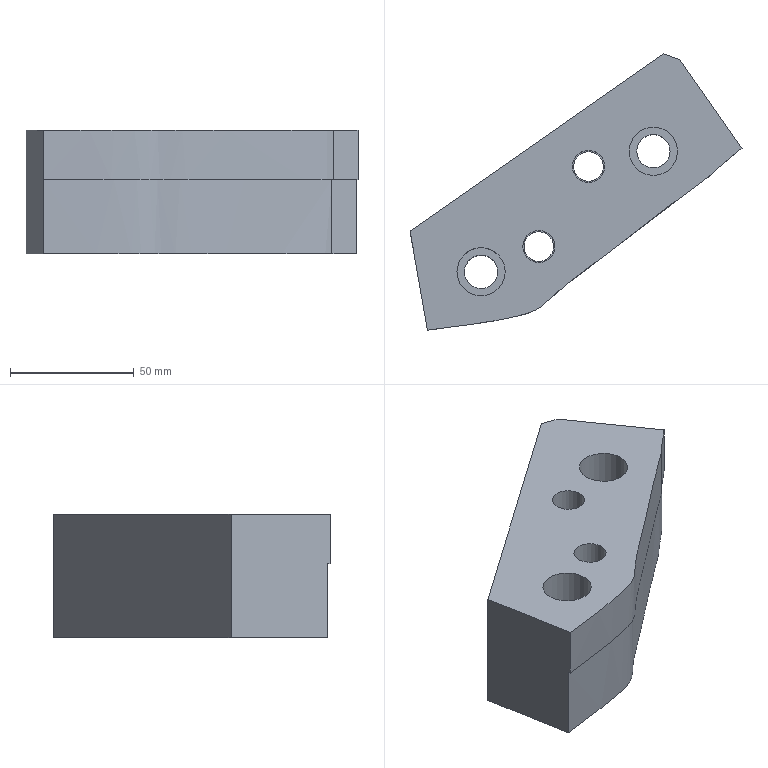Part | NX | features solid 2 | 1 solid | 23 faces | box 134.129 x 111.662 x 50 mm | volume 319985 mm3 | plane 13 | cylinder 8 | spline 2 | commonest cylinder face diameters 12 x2 13 x2 13.5 x2 19.5 x2
STEP:
#1=CARTESIAN_POINT('',(397.794,3.938,0.));
#2=VERTEX_POINT('',#1);
#3=CARTESIAN_POINT('',(397.794,3.938,-20.));
#4=VERTEX_POINT('',#3);
#5=CARTESIAN_POINT('',(397.794,3.938,-10.));
#6=DIRECTION('',(0.,0.,-1.));
#7=VECTOR('',#6,1000.);
#8=LINE('',#5,#7);
#9=EDGE_CURVE('',#2,#4,#8,.T.);
#10=ORIENTED_EDGE('',*,*,#9,.F.);
#11=CARTESIAN_POINT('',(280.528,-61.349,0.));
#12=VERTEX_POINT('',#11);
#13=CARTESIAN_POINT('',(397.794,3.938,0.));
#14=CARTESIAN_POINT('',(396.897,2.818,0.));
#15=CARTESIAN_POINT('',(394.657,0.9582,0.));
#16=CARTESIAN_POINT('',(391.166,-1.547,0.));
#17=CARTESIAN_POINT('',(387.681,-4.089,0.));
#18=CARTESIAN_POINT('',(383.042,-7.479,0.));
#19=CARTESIAN_POINT('',(377.298,-11.791,0.));
#20=CARTESIAN_POINT('',(370.456,-17.031,0.));
#21=CARTESIAN_POINT('',(363.642,-22.308,0.));
#22=CARTESIAN_POINT('',(356.835,-27.594,0.));
#23=CARTESIAN_POINT('',(350.02,-32.87,0.));
#24=CARTESIAN_POINT('',(344.299,-37.211,0.));
#25=CARTESIAN_POINT('',(339.673,-40.62,0.));
#26=CARTESIAN_POINT('',(336.169,-43.134,0.));
#27=CARTESIAN_POINT('',(332.961,-46.001,0.));
#28=CARTESIAN_POINT('',(329.879,-49.024,0.));
#29=CARTESIAN_POINT('',(326.665,-51.86,0.));
#30=CARTESIAN_POINT('',(322.954,-54.002,0.));
#31=CARTESIAN_POINT('',(318.75,-55.232,0.));
#32=CARTESIAN_POINT('',(314.576,-56.215,0.));
#33=CARTESIAN_POINT('',(310.363,-57.101,0.));
#34=CARTESIAN_POINT('',(304.716,-58.092,0.));
#35=CARTESIAN_POINT('',(297.617,-59.134,0.));
#36=CARTESIAN_POINT('',(289.07,-60.222,0.));
#37=CARTESIAN_POINT('',(283.374,-60.967,0.));
#38=CARTESIAN_POINT('',(280.528,-61.349,0.));
#39=B_SPLINE_CURVE_WITH_KNOTS('',3,(#13,#14,#15,#16,#17,#18,#19,#20,#21,#22,#23,#24,#25,#26,#27,#28,#29,#30,#31,#32,#33,#34,#35,#36,#37,#38),.UNSPECIFIED.,.F.,.F.,(4,1,1,1,1,1,1,1,1,1,1,1,1,1,1,1,1,1,1,1,1,1,1,4),(-0.08488,-0.08063,-0.07637,-0.07212,-0.06787,-0.05936,-0.05085,-0.04234,-0.03384,-0.02533,-0.01682,-0.01257,-0.008314,-0.004061,0.0001929,0.004447,0.0087,0.01295,0.01721,0.02146,0.02571,0.03422,0.04273,0.05124),.UNSPECIFIED.);
#40=EDGE_CURVE('',#2,#12,#39,.T.);
#41=ORIENTED_EDGE('',*,*,#40,.T.);
#42=CARTESIAN_POINT('',(280.528,-61.349,-20.));
#43=VERTEX_POINT('',#42);
#44=CARTESIAN_POINT('',(280.528,-61.349,-10.));
#45=DIRECTION('',(0.,0.,-1.));
#46=VECTOR('',#45,1000.);
#47=LINE('',#44,#46);
#48=EDGE_CURVE('',#12,#43,#47,.T.);
#49=ORIENTED_EDGE('',*,*,#48,.T.);
#50=CARTESIAN_POINT('',(-190.231,-121.49,-20.));
#51=CARTESIAN_POINT('',(-188.654,-121.152,-20.));
#52=CARTESIAN_POINT('',(-185.47,-120.627,-20.));
#53=CARTESIAN_POINT('',(-180.656,-120.141,-20.));
#54=CARTESIAN_POINT('',(-175.882,-119.326,-20.));
#55=CARTESIAN_POINT('',(-169.679,-117.528,-20.));
#56=CARTESIAN_POINT('',(-162.185,-114.539,-20.));
#57=CARTESIAN_POINT('',(-153.086,-111.254,-20.));
#58=CARTESIAN_POINT('',(-144.031,-107.845,-20.));
#59=CARTESIAN_POINT('',(-136.465,-105.061,-20.));
#60=CARTESIAN_POINT('',(-130.418,-102.814,-20.));
#61=CARTESIAN_POINT('',(-125.812,-101.329,-20.));
#62=CARTESIAN_POINT('',(-121.306,-99.566,-20.));
#63=CARTESIAN_POINT('',(-116.876,-97.626,-20.));
#64=CARTESIAN_POINT('',(-112.335,-95.923,-20.));
#65=CARTESIAN_POINT('',(-107.564,-95.05,-20.));
#66=CARTESIAN_POINT('',(-102.756,-94.525,-20.));
#67=CARTESIAN_POINT('',(-96.349,-93.771,-20.));
#68=CARTESIAN_POINT('',(-89.902,-93.468,-20.));
#69=CARTESIAN_POINT('',(-83.452,-93.448,-20.));
#70=CARTESIAN_POINT('',(-77.002,-93.469,-20.));
#71=CARTESIAN_POINT('',(-68.939,-93.411,-20.));
#72=CARTESIAN_POINT('',(-56.04,-93.3,-20.));
#73=CARTESIAN_POINT('',(-33.465,-93.184,-20.));
#74=CARTESIAN_POINT('',(-7.666,-93.074,-20.));
#75=CARTESIAN_POINT('',(14.907,-92.653,-20.));
#76=CARTESIAN_POINT('',(27.794,-92.068,-20.));
#77=CARTESIAN_POINT('',(40.668,-91.245,-20.));
#78=CARTESIAN_POINT('',(51.917,-90.291,-20.));
#79=CARTESIAN_POINT('',(61.528,-89.174,-20.));
#80=CARTESIAN_POINT('',(67.939,-88.466,-20.));
#81=CARTESIAN_POINT('',(79.125,-86.95,-20.));
#82=CARTESIAN_POINT('',(95.161,-85.253,-20.));
#83=CARTESIAN_POINT('',(114.404,-83.21,-20.));
#84=CARTESIAN_POINT('',(133.568,-80.524,-20.));
#85=CARTESIAN_POINT('',(152.734,-77.861,-20.));
#86=CARTESIAN_POINT('',(171.916,-75.326,-20.));
#87=CARTESIAN_POINT('',(191.055,-72.413,-20.));
#88=CARTESIAN_POINT('',(207.17,-71.468,-20.));
#89=CARTESIAN_POINT('',(219.951,-69.697,-20.));
#90=CARTESIAN_POINT('',(232.724,-67.899,-20.));
#91=CARTESIAN_POINT('',(248.708,-65.766,-20.));
#92=CARTESIAN_POINT('',(267.87,-63.074,-20.));
#93=CARTESIAN_POINT('',(287.038,-60.44,-20.));
#94=CARTESIAN_POINT('',(301.448,-58.682,-20.));
#95=CARTESIAN_POINT('',(310.976,-56.987,-20.));
#96=CARTESIAN_POINT('',(314.916,-56.135,-20.));
#97=CARTESIAN_POINT('',(318.052,-55.382,-20.));
#98=CARTESIAN_POINT('',(320.39,-54.76,-20.));
#99=CARTESIAN_POINT('',(322.686,-53.981,-20.));
#100=CARTESIAN_POINT('',(325.595,-52.578,-20.));
#101=CARTESIAN_POINT('',(328.769,-50.098,-20.));
#102=CARTESIAN_POINT('',(332.247,-46.69,-20.));
#103=CARTESIAN_POINT('',(335.795,-43.406,-20.));
#104=CARTESIAN_POINT('',(343.661,-37.758,-20.));
#105=CARTESIAN_POINT('',(355.164,-28.914,-20.));
#106=CARTESIAN_POINT('',(370.422,-17.018,-20.));
#107=CARTESIAN_POINT('',(383.264,-7.249,-20.));
#108=CARTESIAN_POINT('',(392.416,-0.6713,-20.));
#109=CARTESIAN_POINT('',(396.953,2.733,-20.));
#110=CARTESIAN_POINT('',(398.886,5.372,-20.));
#111=CARTESIAN_POINT('',(399.725,7.654,-20.));
#112=CARTESIAN_POINT('',(399.76,10.078,-20.));
#113=CARTESIAN_POINT('',(399.483,13.317,-20.));
#114=CARTESIAN_POINT('',(399.712,17.34,-20.));
#115=CARTESIAN_POINT('',(399.612,22.179,-20.));
#116=CARTESIAN_POINT('',(399.633,31.854,-20.));
#117=CARTESIAN_POINT('',(399.593,46.366,-20.));
#118=CARTESIAN_POINT('',(399.637,62.491,-20.));
#119=CARTESIAN_POINT('',(399.588,73.779,-20.));
#120=CARTESIAN_POINT('',(399.652,79.422,-20.));
#121=CARTESIAN_POINT('',(399.59,82.647,-20.));
#122=CARTESIAN_POINT('',(399.564,85.065,-20.));
#123=CARTESIAN_POINT('',(399.725,87.486,-20.));
#124=CARTESIAN_POINT('',(399.756,89.902,-20.));
#125=CARTESIAN_POINT('',(399.247,92.301,-20.));
#126=CARTESIAN_POINT('',(397.362,95.008,-20.));
#127=CARTESIAN_POINT('',(393.635,96.774,-20.));
#128=CARTESIAN_POINT('',(389.279,98.826,-20.));
#129=CARTESIAN_POINT('',(384.732,100.498,-20.));
#130=CARTESIAN_POINT('',(378.765,102.95,-20.));
#131=CARTESIAN_POINT('',(362.589,110.229,-20.));
#132=CARTESIAN_POINT('',(344.928,118.135,-20.));
#133=CARTESIAN_POINT('',(327.281,126.072,-20.));
#134=CARTESIAN_POINT('',(319.932,129.381,-20.));
#135=CARTESIAN_POINT('',(314.075,132.102,-20.));
#136=CARTESIAN_POINT('',(309.387,133.376,-20.));
#137=CARTESIAN_POINT('',(304.547,133.785,-20.));
#138=CARTESIAN_POINT('',(299.716,133.401,-20.));
#139=CARTESIAN_POINT('',(294.929,132.704,-20.));
#140=CARTESIAN_POINT('',(288.543,131.8,-20.));
#141=CARTESIAN_POINT('',(277.364,130.241,-20.));
#142=CARTESIAN_POINT('',(242.2,125.552,-20.));
#143=CARTESIAN_POINT('',(184.637,118.048,-20.));
#144=CARTESIAN_POINT('',(120.701,109.541,-20.));
#145=CARTESIAN_POINT('',(69.531,102.902,-20.));
#146=CARTESIAN_POINT('',(40.777,98.94,-20.));
#147=CARTESIAN_POINT('',(21.566,96.615,-20.));
#148=CARTESIAN_POINT('',(8.743,95.212,-20.));
#149=CARTESIAN_POINT('',(-7.301,93.575,-20.));
#150=CARTESIAN_POINT('',(-26.625,92.505,-20.));
#151=CARTESIAN_POINT('',(-45.971,92.017,-20.));
#152=CARTESIAN_POINT('',(-62.09,91.675,-20.));
#153=CARTESIAN_POINT('',(-74.987,91.256,-20.));
#154=CARTESIAN_POINT('',(-84.664,91.165,-20.));
#155=CARTESIAN_POINT('',(-94.319,91.781,-20.));
#156=CARTESIAN_POINT('',(-103.929,92.966,-20.));
#157=CARTESIAN_POINT('',(-113.495,94.403,-20.));
#158=CARTESIAN_POINT('',(-119.856,95.492,-20.));
#159=CARTESIAN_POINT('',(-122.997,96.222,-20.));
#160=B_SPLINE_CURVE_WITH_KNOTS('',3,(#50,#51,#52,#53,#54,#55,#56,#57,#58,#59,#60,#61,#62,#63,#64,#65,#66,#67,#68,#69,#70,#71,#72,#73,#74,#75,#76,#77,#78,#79,#80,#81,#82,#83,#84,#85,#86,#87,#88,#89,#90,#91,#92,#93,#94,#95,#96,#97,#98,#99,#100,#101,#102,#103,#104,#105,#106,#107,#108,#109,#110,#111,#112,#113,#114,#115,#116,#117,#118,#119,#120,#121,#122,#123,#124,#125,#126,#127,#128,#129,#130,#131,#132,#133,#134,#135,#136,#137,#138,#139,#140,#141,#142,#143,#144,#145,#146,#147,#148,#149,#150,#151,#152,#153,#154,#155,#156,#157,#158,#159),.UNSPECIFIED.,.F.,.F.,(4,1,1,1,1,1,1,1,1,1,1,1,1,1,1,1,1,1,1,1,1,1,1,1,1,1,1,1,1,1,1,1,1,1,1,1,1,1,1,1,1,1,1,1,1,1,1,1,1,1,1,1,1,1,1,1,1,1,1,1,1,1,1,1,1,1,1,1,1,1,1,1,1,1,1,1,1,1,1,1,1,1,1,1,1,1,1,1,1,1,1,1,1,1,1,1,1,1,1,1,1,1,1,1,1,1,1,4),(0.4704,0.4724,0.4745,0.4766,0.4786,0.4828,0.4869,0.491,0.4952,0.4972,0.4993,0.5014,0.5035,0.5055,0.5076,0.5097,0.5117,0.5159,0.5179,0.52,0.5241,0.5283,0.5366,0.5531,0.5614,0.5655,0.5697,0.5779,0.58,0.5821,0.5862,0.5945,0.6028,0.611,0.6193,0.6276,0.6359,0.6441,0.6483,0.6524,0.6607,0.669,0.6772,0.6855,0.6876,0.6897,0.6907,0.6917,0.6928,0.6938,0.6959,0.6979,0.7,0.7021,0.7103,0.7186,0.7269,0.731,0.7331,0.7341,0.7352,0.7362,0.7372,0.7393,0.7414,0.7435,0.7517,0.76,0.7641,0.7662,0.7672,0.7683,0.7693,0.7703,0.7714,0.7724,0.7745,0.7766,0.7786,0.7807,0.7848,0.8014,0.8055,0.8097,0.8117,0.8138,0.8159,0.8179,0.82,0.8221,0.8262,0.8345,0.8676,0.9007,0.9172,0.9338,0.9379,0.9421,0.9503,0.9586,0.9669,0.9752,0.9793,0.9834,0.9876,0.9917,0.9959,1.),.UNSPECIFIED.);
#161=EDGE_CURVE('',#43,#4,#160,.T.);
#162=ORIENTED_EDGE('',*,*,#161,.T.);
#163=EDGE_LOOP('',(#10,#41,#49,#162));
#164=FACE_BOUND('',#163,.T.);
#165=CARTESIAN_POINT('',(280.528,-61.349,0.));
#166=CARTESIAN_POINT('',(280.528,-61.349,-20.));
#167=CARTESIAN_POINT('',(283.373,-60.967,0.));
#168=CARTESIAN_POINT('',(283.373,-60.967,-20.));
#169=CARTESIAN_POINT('',(289.068,-60.222,0.));
#170=CARTESIAN_POINT('',(289.068,-60.222,-20.));
#171=CARTESIAN_POINT('',(297.614,-59.134,0.));
#172=CARTESIAN_POINT('',(297.614,-59.134,-20.));
#173=CARTESIAN_POINT('',(304.716,-58.093,0.));
#174=CARTESIAN_POINT('',(304.716,-58.093,-20.));
#175=CARTESIAN_POINT('',(310.373,-57.099,0.));
#176=CARTESIAN_POINT('',(310.373,-57.099,-20.));
#177=CARTESIAN_POINT('',(314.589,-56.213,0.));
#178=CARTESIAN_POINT('',(314.589,-56.213,-20.));
#179=CARTESIAN_POINT('',(318.776,-55.225,0.));
#180=CARTESIAN_POINT('',(318.776,-55.225,-20.));
#181=CARTESIAN_POINT('',(322.935,-54.009,0.));
#182=CARTESIAN_POINT('',(322.935,-54.009,-20.));
#183=CARTESIAN_POINT('',(326.673,-51.857,0.));
#184=CARTESIAN_POINT('',(326.673,-51.857,-20.));
#185=CARTESIAN_POINT('',(329.907,-48.998,0.));
#186=CARTESIAN_POINT('',(329.907,-48.998,-20.));
#187=CARTESIAN_POINT('',(332.997,-45.965,0.));
#188=CARTESIAN_POINT('',(332.997,-45.965,-20.));
#189=CARTESIAN_POINT('',(336.207,-43.104,0.));
#190=CARTESIAN_POINT('',(336.207,-43.104,-20.));
#191=CARTESIAN_POINT('',(339.712,-40.593,0.));
#192=CARTESIAN_POINT('',(339.712,-40.593,-20.));
#193=CARTESIAN_POINT('',(344.335,-37.183,0.));
#194=CARTESIAN_POINT('',(344.335,-37.183,-20.));
#195=CARTESIAN_POINT('',(350.054,-32.844,0.));
#196=CARTESIAN_POINT('',(350.054,-32.844,-20.));
#197=CARTESIAN_POINT('',(356.864,-27.572,0.));
#198=CARTESIAN_POINT('',(356.864,-27.572,-20.));
#199=CARTESIAN_POINT('',(363.666,-22.289,0.));
#200=CARTESIAN_POINT('',(363.666,-22.289,-20.));
#201=CARTESIAN_POINT('',(370.477,-17.014,0.));
#202=CARTESIAN_POINT('',(370.477,-17.014,-20.));
#203=CARTESIAN_POINT('',(377.319,-11.775,0.));
#204=CARTESIAN_POINT('',(377.319,-11.775,-20.));
#205=CARTESIAN_POINT('',(383.06,-7.466,0.));
#206=CARTESIAN_POINT('',(383.06,-7.466,-20.));
#207=CARTESIAN_POINT('',(387.692,-4.081,0.));
#208=CARTESIAN_POINT('',(387.692,-4.081,-20.));
#209=CARTESIAN_POINT('',(391.168,-1.546,0.));
#210=CARTESIAN_POINT('',(391.168,-1.546,-20.));
#211=CARTESIAN_POINT('',(394.677,0.9741,0.));
#212=CARTESIAN_POINT('',(394.677,0.9741,-20.));
#213=CARTESIAN_POINT('',(396.893,2.813,0.));
#214=CARTESIAN_POINT('',(396.893,2.813,-20.));
#215=CARTESIAN_POINT('',(397.794,3.938,0.));
#216=CARTESIAN_POINT('',(397.794,3.938,-20.));
#217=B_SPLINE_SURFACE_WITH_KNOTS('',3,1,((#165,#166),(#167,#168),(#169,#170),(#171,#172),(#173,#174),(#175,#176),(#177,#178),(#179,#180),(#181,#182),(#183,#184),(#185,#186),(#187,#188),(#189,#190),(#191,#192),(#193,#194),(#195,#196),(#197,#198),(#199,#200),(#201,#202),(#203,#204),(#205,#206),(#207,#208),(#209,#210),(#211,#212),(#213,#214),(#215,#216)),.SURF_OF_LINEAR_EXTRUSION.,.F.,.F.,.F.,(4,1,1,1,1,1,1,1,1,1,1,1,1,1,1,1,1,1,1,1,1,1,1,4),(2,2),(0.6744,0.6781,0.6818,0.6855,0.6873,0.6892,0.691,0.6929,0.6947,0.6965,0.6984,0.7002,0.7021,0.7039,0.7076,0.7113,0.715,0.7186,0.7223,0.726,0.7279,0.7297,0.7315,0.7334),(0.,1.),.UNSPECIFIED.);
#218=ADVANCED_FACE('',(#164),#217,.F.);
#219=CARTESIAN_POINT('',(375.7,50.313,-50.));
#220=VERTEX_POINT('',#219);
#221=CARTESIAN_POINT('',(273.462,-21.276,-50.));
#222=VERTEX_POINT('',#221);
#223=CARTESIAN_POINT('',(-162.34,-326.427,-50.));
#224=DIRECTION('',(-0.8192,-0.5736,0.));
#225=VECTOR('',#224,1000.);
#226=LINE('',#223,#225);
#227=EDGE_CURVE('',#220,#222,#226,.T.);
#228=ORIENTED_EDGE('',*,*,#227,.F.);
#229=CARTESIAN_POINT('',(382.644,47.785,-50.));
#230=VERTEX_POINT('',#229);
#231=CARTESIAN_POINT('',(-318.035,302.812,-50.));
#232=DIRECTION('',(0.9397,-0.342,0.));
#233=VECTOR('',#232,1000.);
#234=LINE('',#231,#233);
#235=EDGE_CURVE('',#220,#230,#234,.T.);
#236=ORIENTED_EDGE('',*,*,#235,.T.);
#237=CARTESIAN_POINT('',(407.015,12.981,-50.));
#238=VERTEX_POINT('',#237);
#239=CARTESIAN_POINT('',(126.035,414.261,-50.));
#240=DIRECTION('',(0.5736,-0.8192,0.));
#241=VECTOR('',#240,1000.);
#242=LINE('',#239,#241);
#243=EDGE_CURVE('',#230,#238,#242,.T.);
#244=ORIENTED_EDGE('',*,*,#243,.T.);
#245=CARTESIAN_POINT('',(397.074,4.639,-50.));
#246=VERTEX_POINT('',#245);
#247=CARTESIAN_POINT('',(402.92,9.544,-50.));
#248=DIRECTION('',(-0.766,-0.6428,0.));
#249=VECTOR('',#248,1000.);
#250=LINE('',#247,#249);
#251=EDGE_CURVE('',#238,#246,#250,.T.);
#252=ORIENTED_EDGE('',*,*,#251,.T.);
#253=CARTESIAN_POINT('',(280.354,-60.363,-50.));
#254=VERTEX_POINT('',#253);
#255=CARTESIAN_POINT('',(397.074,4.639,-50.));
#256=CARTESIAN_POINT('',(396.211,3.541,-50.));
#257=CARTESIAN_POINT('',(394.025,1.739,-50.));
#258=CARTESIAN_POINT('',(390.615,-0.7124,-50.));
#259=CARTESIAN_POINT('',(387.212,-3.194,-50.));
#260=CARTESIAN_POINT('',(382.68,-6.503,-50.));
#261=CARTESIAN_POINT('',(377.069,-10.711,-50.));
#262=CARTESIAN_POINT('',(370.384,-15.824,-50.));
#263=CARTESIAN_POINT('',(363.727,-20.975,-50.));
#264=CARTESIAN_POINT('',(357.08,-26.138,-50.));
#265=CARTESIAN_POINT('',(350.428,-31.295,-50.));
#266=CARTESIAN_POINT('',(344.846,-35.541,-50.));
#267=CARTESIAN_POINT('',(340.348,-38.897,-50.));
#268=CARTESIAN_POINT('',(336.918,-41.336,-50.));
#269=CARTESIAN_POINT('',(333.636,-43.987,-50.));
#270=CARTESIAN_POINT('',(329.544,-47.935,-50.));
#271=CARTESIAN_POINT('',(324.416,-52.834,-50.));
#272=CARTESIAN_POINT('',(315.633,-54.99,-50.));
#273=CARTESIAN_POINT('',(306.9,-56.771,-50.));
#274=CARTESIAN_POINT('',(298.061,-58.061,-50.));
#275=CARTESIAN_POINT('',(289.206,-59.198,-50.));
#276=CARTESIAN_POINT('',(283.303,-59.967,-50.));
#277=CARTESIAN_POINT('',(280.354,-60.363,-50.));
#278=B_SPLINE_CURVE_WITH_KNOTS('',3,(#255,#256,#257,#258,#259,#260,#261,#262,#263,#264,#265,#266,#267,#268,#269,#270,#271,#272,#273,#274,#275,#276,#277),.UNSPECIFIED.,.F.,.F.,(4,1,1,1,1,1,1,1,1,1,1,1,1,1,1,1,1,1,1,1,4),(0.03805,0.04226,0.04648,0.05069,0.0549,0.06333,0.07175,0.08018,0.08861,0.09703,0.1055,0.1097,0.1139,0.1181,0.1223,0.1307,0.1392,0.1476,0.156,0.1644,0.1729),.UNSPECIFIED.);
#279=EDGE_CURVE('',#246,#254,#278,.T.);
#280=ORIENTED_EDGE('',*,*,#279,.T.);
#281=CARTESIAN_POINT('',(243.048,151.206,-50.));
#282=DIRECTION('',(-0.1736,0.9848,0.));
#283=VECTOR('',#282,1000.);
#284=LINE('',#281,#283);
#285=EDGE_CURVE('',#254,#222,#284,.T.);
#286=ORIENTED_EDGE('',*,*,#285,.T.);
#287=EDGE_LOOP('',(#228,#236,#244,#252,#280,#286));
#288=FACE_BOUND('',#287,.T.);
#289=CARTESIAN_POINT('',(351.591,4.814,-50.));
#290=VERTEX_POINT('',#289);
#291=CARTESIAN_POINT('',(345.591,4.814,-50.));
#292=DIRECTION('',(0.,0.,1.));
#293=DIRECTION('',(1.,0.,0.));
#294=AXIS2_PLACEMENT_3D('',#291,#292,#293);
#295=CIRCLE('',#294,6.);
#296=EDGE_CURVE('',#290,#290,#295,.T.);
#297=ORIENTED_EDGE('',*,*,#296,.T.);
#298=EDGE_LOOP('',(#297));
#299=FACE_BOUND('',#298,.T.);
#300=CARTESIAN_POINT('',(331.524,-27.549,-50.));
#301=VERTEX_POINT('',#300);
#302=CARTESIAN_POINT('',(325.524,-27.549,-50.));
#303=DIRECTION('',(0.,0.,1.));
#304=DIRECTION('',(1.,0.,0.));
#305=AXIS2_PLACEMENT_3D('',#302,#303,#304);
#306=CIRCLE('',#305,6.);
#307=EDGE_CURVE('',#301,#301,#306,.T.);
#308=ORIENTED_EDGE('',*,*,#307,.T.);
#309=EDGE_LOOP('',(#308));
#310=FACE_BOUND('',#309,.T.);
#311=CARTESIAN_POINT('',(308.927,-37.792,-50.));
#312=VERTEX_POINT('',#311);
#313=CARTESIAN_POINT('',(302.177,-37.792,-50.));
#314=DIRECTION('',(0.,0.,1.));
#315=DIRECTION('',(1.,0.,0.));
#316=AXIS2_PLACEMENT_3D('',#313,#314,#315);
#317=CIRCLE('',#316,6.75);
#318=EDGE_CURVE('',#312,#312,#317,.T.);
#319=ORIENTED_EDGE('',*,*,#318,.T.);
#320=EDGE_LOOP('',(#319));
#321=FACE_BOUND('',#320,.T.);
#322=CARTESIAN_POINT('',(378.555,10.962,-50.));
#323=VERTEX_POINT('',#322);
#324=CARTESIAN_POINT('',(371.805,10.962,-50.));
#325=DIRECTION('',(0.,0.,1.));
#326=DIRECTION('',(1.,0.,0.));
#327=AXIS2_PLACEMENT_3D('',#324,#325,#326);
#328=CIRCLE('',#327,6.75);
#329=EDGE_CURVE('',#323,#323,#328,.T.);
#330=ORIENTED_EDGE('',*,*,#329,.T.);
#331=EDGE_LOOP('',(#330));
#332=FACE_BOUND('',#331,.T.);
#333=CARTESIAN_POINT('',(-415.478,35.09,-50.));
#334=DIRECTION('',(0.,0.,1.));
#335=DIRECTION('',(1.,0.,0.));
#336=AXIS2_PLACEMENT_3D('',#333,#334,#335);
#337=PLANE('',#336);
#338=ADVANCED_FACE('',(#288,#299,#310,#321,#332),#337,.F.);
#339=CARTESIAN_POINT('',(407.591,12.158,0.));
#340=VERTEX_POINT('',#339);
#341=CARTESIAN_POINT('',(382.644,47.785,0.));
#342=VERTEX_POINT('',#341);
#343=CARTESIAN_POINT('',(228.765,267.547,0.));
#344=DIRECTION('',(-0.5736,0.8192,0.));
#345=VECTOR('',#344,1000.);
#346=LINE('',#343,#345);
#347=EDGE_CURVE('',#340,#342,#346,.T.);
#348=ORIENTED_EDGE('',*,*,#347,.T.);
#349=CARTESIAN_POINT('',(375.7,50.313,0.));
#350=VERTEX_POINT('',#349);
#351=CARTESIAN_POINT('',(-283.889,290.383,0.));
#352=DIRECTION('',(-0.9397,0.342,0.));
#353=VECTOR('',#352,1000.);
#354=LINE('',#351,#353);
#355=EDGE_CURVE('',#342,#350,#354,.T.);
#356=ORIENTED_EDGE('',*,*,#355,.T.);
#357=CARTESIAN_POINT('',(273.462,-21.276,0.));
#358=VERTEX_POINT('',#357);
#359=CARTESIAN_POINT('',(-319.974,-436.804,0.));
#360=DIRECTION('',(0.8192,0.5736,0.));
#361=VECTOR('',#360,1000.);
#362=LINE('',#359,#361);
#363=EDGE_CURVE('',#358,#350,#362,.T.);
#364=ORIENTED_EDGE('',*,*,#363,.F.);
#365=CARTESIAN_POINT('',(285.358,-88.743,0.));
#366=DIRECTION('',(0.1736,-0.9848,0.));
#367=VECTOR('',#366,1000.);
#368=LINE('',#365,#367);
#369=EDGE_CURVE('',#358,#12,#368,.T.);
#370=ORIENTED_EDGE('',*,*,#369,.T.);
#371=ORIENTED_EDGE('',*,*,#40,.F.);
#372=CARTESIAN_POINT('',(386.216,-5.777,0.));
#373=DIRECTION('',(0.766,0.6428,0.));
#374=VECTOR('',#373,1000.);
#375=LINE('',#372,#374);
#376=EDGE_CURVE('',#340,#2,#375,.F.);
#377=ORIENTED_EDGE('',*,*,#376,.F.);
#378=EDGE_LOOP('',(#348,#356,#364,#370,#371,#377));
#379=FACE_BOUND('',#378,.T.);
#380=CARTESIAN_POINT('',(362.055,10.962,0.));
#381=VERTEX_POINT('',#380);
#382=CARTESIAN_POINT('',(371.805,10.962,0.));
#383=DIRECTION('',(0.,0.,-1.));
#384=DIRECTION('',(-1.,0.,0.));
#385=AXIS2_PLACEMENT_3D('',#382,#383,#384);
#386=CIRCLE('',#385,9.75);
#387=EDGE_CURVE('',#381,#381,#386,.T.);
#388=ORIENTED_EDGE('',*,*,#387,.T.);
#389=EDGE_LOOP('',(#388));
#390=FACE_BOUND('',#389,.T.);
#391=CARTESIAN_POINT('',(292.427,-37.792,0.));
#392=VERTEX_POINT('',#391);
#393=CARTESIAN_POINT('',(302.177,-37.792,0.));
#394=DIRECTION('',(0.,0.,-1.));
#395=DIRECTION('',(-1.,0.,0.));
#396=AXIS2_PLACEMENT_3D('',#393,#394,#395);
#397=CIRCLE('',#396,9.75);
#398=EDGE_CURVE('',#392,#392,#397,.T.);
#399=ORIENTED_EDGE('',*,*,#398,.T.);
#400=EDGE_LOOP('',(#399));
#401=FACE_BOUND('',#400,.T.);
#402=CARTESIAN_POINT('',(319.024,-27.549,0.));
#403=VERTEX_POINT('',#402);
#404=CARTESIAN_POINT('',(325.524,-27.549,0.));
#405=DIRECTION('',(0.,0.,-1.));
#406=DIRECTION('',(-1.,0.,0.));
#407=AXIS2_PLACEMENT_3D('',#404,#405,#406);
#408=CIRCLE('',#407,6.5);
#409=EDGE_CURVE('',#403,#403,#408,.T.);
#410=ORIENTED_EDGE('',*,*,#409,.T.);
#411=EDGE_LOOP('',(#410));
#412=FACE_BOUND('',#411,.T.);
#413=CARTESIAN_POINT('',(339.091,4.814,0.));
#414=VERTEX_POINT('',#413);
#415=CARTESIAN_POINT('',(345.591,4.814,0.));
#416=DIRECTION('',(0.,0.,-1.));
#417=DIRECTION('',(-1.,0.,0.));
#418=AXIS2_PLACEMENT_3D('',#415,#416,#417);
#419=CIRCLE('',#418,6.5);
#420=EDGE_CURVE('',#414,#414,#419,.T.);
#421=ORIENTED_EDGE('',*,*,#420,.T.);
#422=EDGE_LOOP('',(#421));
#423=FACE_BOUND('',#422,.T.);
#424=CARTESIAN_POINT('',(-470.381,-222.,0.));
#425=DIRECTION('',(0.,0.,-1.));
#426=DIRECTION('',(-1.,0.,0.));
#427=AXIS2_PLACEMENT_3D('',#424,#425,#426);
#428=PLANE('',#427);
#429=ADVANCED_FACE('',(#379,#390,#401,#412,#423),#428,.F.);
#430=ORIENTED_EDGE('',*,*,#243,.F.);
#431=CARTESIAN_POINT('',(382.644,47.785,0.));
#432=DIRECTION('',(0.,0.,1.));
#433=VECTOR('',#432,1000.);
#434=LINE('',#431,#433);
#435=EDGE_CURVE('',#230,#342,#434,.T.);
#436=ORIENTED_EDGE('',*,*,#435,.T.);
#437=ORIENTED_EDGE('',*,*,#347,.F.);
#438=CARTESIAN_POINT('',(407.591,12.158,-20.));
#439=VERTEX_POINT('',#438);
#440=CARTESIAN_POINT('',(407.591,12.158,100.));
#441=DIRECTION('',(0.,0.,1.));
#442=VECTOR('',#441,1000.);
#443=LINE('',#440,#442);
#444=EDGE_CURVE('',#439,#340,#443,.T.);
#445=ORIENTED_EDGE('',*,*,#444,.F.);
#446=CARTESIAN_POINT('',(407.015,12.981,-20.));
#447=VERTEX_POINT('',#446);
#448=CARTESIAN_POINT('',(342.17,105.589,-20.));
#449=DIRECTION('',(-0.5736,0.8192,0.));
#450=VECTOR('',#449,1000.);
#451=LINE('',#448,#450);
#452=EDGE_CURVE('',#439,#447,#451,.T.);
#453=ORIENTED_EDGE('',*,*,#452,.T.);
#454=CARTESIAN_POINT('',(407.015,12.981,-20.));
#455=DIRECTION('',(0.,0.,-1.));
#456=VECTOR('',#455,1000.);
#457=LINE('',#454,#456);
#458=EDGE_CURVE('',#447,#238,#457,.T.);
#459=ORIENTED_EDGE('',*,*,#458,.T.);
#460=EDGE_LOOP('',(#430,#436,#437,#445,#453,#459));
#461=FACE_BOUND('',#460,.T.);
#462=CARTESIAN_POINT('',(342.17,105.589,0.));
#463=DIRECTION('',(-0.8192,-0.5736,0.));
#464=DIRECTION('',(0.5736,-0.8192,0.));
#465=AXIS2_PLACEMENT_3D('',#462,#463,#464);
#466=PLANE('',#465);
#467=ADVANCED_FACE('',(#461),#466,.F.);
#468=CARTESIAN_POINT('',(375.7,50.313,0.));
#469=DIRECTION('',(0.,0.,1.));
#470=VECTOR('',#469,1000.);
#471=LINE('',#468,#470);
#472=EDGE_CURVE('',#220,#350,#471,.T.);
#473=ORIENTED_EDGE('',*,*,#472,.F.);
#474=ORIENTED_EDGE('',*,*,#227,.T.);
#475=CARTESIAN_POINT('',(273.462,-21.276,0.));
#476=DIRECTION('',(0.,0.,-1.));
#477=VECTOR('',#476,1000.);
#478=LINE('',#475,#477);
#479=EDGE_CURVE('',#358,#222,#478,.T.);
#480=ORIENTED_EDGE('',*,*,#479,.F.);
#481=ORIENTED_EDGE('',*,*,#363,.T.);
#482=EDGE_LOOP('',(#473,#474,#480,#481));
#483=FACE_BOUND('',#482,.T.);
#484=CARTESIAN_POINT('',(375.077,49.876,0.));
#485=DIRECTION('',(-0.5736,0.8192,0.));
#486=DIRECTION('',(-0.8192,-0.5736,0.));
#487=AXIS2_PLACEMENT_3D('',#484,#485,#486);
#488=PLANE('',#487);
#489=ADVANCED_FACE('',(#483),#488,.T.);
#490=CARTESIAN_POINT('',(280.354,-60.363,-20.));
#491=VERTEX_POINT('',#490);
#492=CARTESIAN_POINT('',(280.354,-60.363,-60.));
#493=DIRECTION('',(0.,0.,-1.));
#494=VECTOR('',#493,1000.);
#495=LINE('',#492,#494);
#496=EDGE_CURVE('',#254,#491,#495,.F.);
#497=ORIENTED_EDGE('',*,*,#496,.T.);
#498=CARTESIAN_POINT('',(298.119,-161.113,-20.));
#499=DIRECTION('',(0.1736,-0.9848,0.));
#500=VECTOR('',#499,1000.);
#501=LINE('',#498,#500);
#502=EDGE_CURVE('',#491,#43,#501,.T.);
#503=ORIENTED_EDGE('',*,*,#502,.T.);
#504=ORIENTED_EDGE('',*,*,#48,.F.);
#505=ORIENTED_EDGE('',*,*,#369,.F.);
#506=ORIENTED_EDGE('',*,*,#479,.T.);
#507=ORIENTED_EDGE('',*,*,#285,.F.);
#508=EDGE_LOOP('',(#497,#503,#504,#505,#506,#507));
#509=FACE_BOUND('',#508,.T.);
#510=CARTESIAN_POINT('',(298.119,-161.113,0.));
#511=DIRECTION('',(0.9848,0.1736,0.));
#512=DIRECTION('',(-0.1736,0.9848,0.));
#513=AXIS2_PLACEMENT_3D('',#510,#511,#512);
#514=PLANE('',#513);
#515=ADVANCED_FACE('',(#509),#514,.F.);
#516=CARTESIAN_POINT('',(365.055,10.962,-15.));
#517=VERTEX_POINT('',#516);
#518=CARTESIAN_POINT('',(371.805,10.962,-15.));
#519=DIRECTION('',(0.,0.,-1.));
#520=DIRECTION('',(-1.,0.,0.));
#521=AXIS2_PLACEMENT_3D('',#518,#519,#520);
#522=CIRCLE('',#521,6.75);
#523=EDGE_CURVE('',#517,#517,#522,.T.);
#524=ORIENTED_EDGE('',*,*,#523,.F.);
#525=EDGE_LOOP('',(#524));
#526=FACE_BOUND('',#525,.T.);
#527=ORIENTED_EDGE('',*,*,#329,.F.);
#528=EDGE_LOOP('',(#527));
#529=FACE_BOUND('',#528,.T.);
#530=CARTESIAN_POINT('',(371.805,10.962,-100.));
#531=DIRECTION('',(0.,0.,-1.));
#532=DIRECTION('',(-1.,0.,0.));
#533=AXIS2_PLACEMENT_3D('',#530,#531,#532);
#534=CYLINDRICAL_SURFACE('',#533,6.75);
#535=ADVANCED_FACE('',(#526,#529),#534,.F.);
#536=ORIENTED_EDGE('',*,*,#523,.T.);
#537=EDGE_LOOP('',(#536));
#538=FACE_BOUND('',#537,.T.);
#539=CARTESIAN_POINT('',(362.055,10.962,-15.));
#540=VERTEX_POINT('',#539);
#541=CARTESIAN_POINT('',(371.805,10.962,-15.));
#542=DIRECTION('',(0.,0.,-1.));
#543=DIRECTION('',(-1.,0.,0.));
#544=AXIS2_PLACEMENT_3D('',#541,#542,#543);
#545=CIRCLE('',#544,9.75);
#546=EDGE_CURVE('',#540,#540,#545,.T.);
#547=ORIENTED_EDGE('',*,*,#546,.F.);
#548=EDGE_LOOP('',(#547));
#549=FACE_BOUND('',#548,.T.);
#550=CARTESIAN_POINT('',(371.805,10.962,-15.));
#551=DIRECTION('',(0.,0.,-1.));
#552=DIRECTION('',(-1.,0.,0.));
#553=AXIS2_PLACEMENT_3D('',#550,#551,#552);
#554=PLANE('',#553);
#555=ADVANCED_FACE('',(#538,#549),#554,.F.);
#556=ORIENTED_EDGE('',*,*,#546,.T.);
#557=EDGE_LOOP('',(#556));
#558=FACE_BOUND('',#557,.T.);
#559=ORIENTED_EDGE('',*,*,#387,.F.);
#560=EDGE_LOOP('',(#559));
#561=FACE_BOUND('',#560,.T.);
#562=CARTESIAN_POINT('',(371.805,10.962,0.));
#563=DIRECTION('',(0.,0.,-1.));
#564=DIRECTION('',(-1.,0.,0.));
#565=AXIS2_PLACEMENT_3D('',#562,#563,#564);
#566=CYLINDRICAL_SURFACE('',#565,9.75);
#567=ADVANCED_FACE('',(#558,#561),#566,.F.);
#568=CARTESIAN_POINT('',(295.427,-37.792,-15.));
#569=VERTEX_POINT('',#568);
#570=CARTESIAN_POINT('',(302.177,-37.792,-15.));
#571=DIRECTION('',(0.,0.,-1.));
#572=DIRECTION('',(-1.,0.,0.));
#573=AXIS2_PLACEMENT_3D('',#570,#571,#572);
#574=CIRCLE('',#573,6.75);
#575=EDGE_CURVE('',#569,#569,#574,.T.);
#576=ORIENTED_EDGE('',*,*,#575,.F.);
#577=EDGE_LOOP('',(#576));
#578=FACE_BOUND('',#577,.T.);
#579=ORIENTED_EDGE('',*,*,#318,.F.);
#580=EDGE_LOOP('',(#579));
#581=FACE_BOUND('',#580,.T.);
#582=CARTESIAN_POINT('',(302.177,-37.792,-100.));
#583=DIRECTION('',(0.,0.,-1.));
#584=DIRECTION('',(-1.,0.,0.));
#585=AXIS2_PLACEMENT_3D('',#582,#583,#584);
#586=CYLINDRICAL_SURFACE('',#585,6.75);
#587=ADVANCED_FACE('',(#578,#581),#586,.F.);
#588=ORIENTED_EDGE('',*,*,#575,.T.);
#589=EDGE_LOOP('',(#588));
#590=FACE_BOUND('',#589,.T.);
#591=CARTESIAN_POINT('',(292.427,-37.792,-15.));
#592=VERTEX_POINT('',#591);
#593=CARTESIAN_POINT('',(302.177,-37.792,-15.));
#594=DIRECTION('',(0.,0.,-1.));
#595=DIRECTION('',(-1.,0.,0.));
#596=AXIS2_PLACEMENT_3D('',#593,#594,#595);
#597=CIRCLE('',#596,9.75);
#598=EDGE_CURVE('',#592,#592,#597,.T.);
#599=ORIENTED_EDGE('',*,*,#598,.F.);
#600=EDGE_LOOP('',(#599));
#601=FACE_BOUND('',#600,.T.);
#602=CARTESIAN_POINT('',(302.177,-37.792,-15.));
#603=DIRECTION('',(0.,0.,-1.));
#604=DIRECTION('',(-1.,0.,0.));
#605=AXIS2_PLACEMENT_3D('',#602,#603,#604);
#606=PLANE('',#605);
#607=ADVANCED_FACE('',(#590,#601),#606,.F.);
#608=ORIENTED_EDGE('',*,*,#598,.T.);
#609=EDGE_LOOP('',(#608));
#610=FACE_BOUND('',#609,.T.);
#611=ORIENTED_EDGE('',*,*,#398,.F.);
#612=EDGE_LOOP('',(#611));
#613=FACE_BOUND('',#612,.T.);
#614=CARTESIAN_POINT('',(302.177,-37.792,0.));
#615=DIRECTION('',(0.,0.,-1.));
#616=DIRECTION('',(-1.,0.,0.));
#617=AXIS2_PLACEMENT_3D('',#614,#615,#616);
#618=CYLINDRICAL_SURFACE('',#617,9.75);
#619=ADVANCED_FACE('',(#610,#613),#618,.F.);
#620=CARTESIAN_POINT('',(319.524,-27.549,-20.));
#621=VERTEX_POINT('',#620);
#622=CARTESIAN_POINT('',(325.524,-27.549,-20.));
#623=DIRECTION('',(0.,0.,-1.));
#624=DIRECTION('',(-1.,0.,0.));
#625=AXIS2_PLACEMENT_3D('',#622,#623,#624);
#626=CIRCLE('',#625,6.);
#627=EDGE_CURVE('',#621,#621,#626,.T.);
#628=ORIENTED_EDGE('',*,*,#627,.F.);
#629=EDGE_LOOP('',(#628));
#630=FACE_BOUND('',#629,.T.);
#631=ORIENTED_EDGE('',*,*,#307,.F.);
#632=EDGE_LOOP('',(#631));
#633=FACE_BOUND('',#632,.T.);
#634=CARTESIAN_POINT('',(325.524,-27.549,-100.));
#635=DIRECTION('',(0.,0.,-1.));
#636=DIRECTION('',(-1.,0.,0.));
#637=AXIS2_PLACEMENT_3D('',#634,#635,#636);
#638=CYLINDRICAL_SURFACE('',#637,6.);
#639=ADVANCED_FACE('',(#630,#633),#638,.F.);
#640=ORIENTED_EDGE('',*,*,#627,.T.);
#641=EDGE_LOOP('',(#640));
#642=FACE_BOUND('',#641,.T.);
#643=CARTESIAN_POINT('',(319.024,-27.549,-20.));
#644=VERTEX_POINT('',#643);
#645=CARTESIAN_POINT('',(325.524,-27.549,-20.));
#646=DIRECTION('',(0.,0.,-1.));
#647=DIRECTION('',(-1.,0.,0.));
#648=AXIS2_PLACEMENT_3D('',#645,#646,#647);
#649=CIRCLE('',#648,6.5);
#650=EDGE_CURVE('',#644,#644,#649,.T.);
#651=ORIENTED_EDGE('',*,*,#650,.F.);
#652=EDGE_LOOP('',(#651));
#653=FACE_BOUND('',#652,.T.);
#654=CARTESIAN_POINT('',(325.524,-27.549,-20.));
#655=DIRECTION('',(0.,0.,-1.));
#656=DIRECTION('',(-1.,0.,0.));
#657=AXIS2_PLACEMENT_3D('',#654,#655,#656);
#658=PLANE('',#657);
#659=ADVANCED_FACE('',(#642,#653),#658,.F.);
#660=ORIENTED_EDGE('',*,*,#650,.T.);
#661=EDGE_LOOP('',(#660));
#662=FACE_BOUND('',#661,.T.);
#663=ORIENTED_EDGE('',*,*,#409,.F.);
#664=EDGE_LOOP('',(#663));
#665=FACE_BOUND('',#664,.T.);
#666=CARTESIAN_POINT('',(325.524,-27.549,0.));
#667=DIRECTION('',(0.,0.,-1.));
#668=DIRECTION('',(-1.,0.,0.));
#669=AXIS2_PLACEMENT_3D('',#666,#667,#668);
#670=CYLINDRICAL_SURFACE('',#669,6.5);
#671=ADVANCED_FACE('',(#662,#665),#670,.F.);
#672=CARTESIAN_POINT('',(339.591,4.814,-20.));
#673=VERTEX_POINT('',#672);
#674=CARTESIAN_POINT('',(345.591,4.814,-20.));
#675=DIRECTION('',(0.,0.,-1.));
#676=DIRECTION('',(-1.,0.,0.));
#677=AXIS2_PLACEMENT_3D('',#674,#675,#676);
#678=CIRCLE('',#677,6.);
#679=EDGE_CURVE('',#673,#673,#678,.T.);
#680=ORIENTED_EDGE('',*,*,#679,.F.);
#681=EDGE_LOOP('',(#680));
#682=FACE_BOUND('',#681,.T.);
#683=ORIENTED_EDGE('',*,*,#296,.F.);
#684=EDGE_LOOP('',(#683));
#685=FACE_BOUND('',#684,.T.);
#686=CARTESIAN_POINT('',(345.591,4.814,-100.));
#687=DIRECTION('',(0.,0.,-1.));
#688=DIRECTION('',(-1.,0.,0.));
#689=AXIS2_PLACEMENT_3D('',#686,#687,#688);
#690=CYLINDRICAL_SURFACE('',#689,6.);
#691=ADVANCED_FACE('',(#682,#685),#690,.F.);
#692=ORIENTED_EDGE('',*,*,#679,.T.);
#693=EDGE_LOOP('',(#692));
#694=FACE_BOUND('',#693,.T.);
#695=CARTESIAN_POINT('',(339.091,4.814,-20.));
#696=VERTEX_POINT('',#695);
#697=CARTESIAN_POINT('',(345.591,4.814,-20.));
#698=DIRECTION('',(0.,0.,-1.));
#699=DIRECTION('',(-1.,0.,0.));
#700=AXIS2_PLACEMENT_3D('',#697,#698,#699);
#701=CIRCLE('',#700,6.5);
#702=EDGE_CURVE('',#696,#696,#701,.T.);
#703=ORIENTED_EDGE('',*,*,#702,.F.);
#704=EDGE_LOOP('',(#703));
#705=FACE_BOUND('',#704,.T.);
#706=CARTESIAN_POINT('',(348.458,0.7182,-20.));
#707=DIRECTION('',(0.,0.,-1.));
#708=DIRECTION('',(-1.,0.,0.));
#709=AXIS2_PLACEMENT_3D('',#706,#707,#708);
#710=PLANE('',#709);
#711=ADVANCED_FACE('',(#694,#705),#710,.F.);
#712=ORIENTED_EDGE('',*,*,#702,.T.);
#713=EDGE_LOOP('',(#712));
#714=FACE_BOUND('',#713,.T.);
#715=ORIENTED_EDGE('',*,*,#420,.F.);
#716=EDGE_LOOP('',(#715));
#717=FACE_BOUND('',#716,.T.);
#718=CARTESIAN_POINT('',(345.591,4.814,0.));
#719=DIRECTION('',(0.,0.,-1.));
#720=DIRECTION('',(-1.,0.,0.));
#721=AXIS2_PLACEMENT_3D('',#718,#719,#720);
#722=CYLINDRICAL_SURFACE('',#721,6.5);
#723=ADVANCED_FACE('',(#714,#717),#722,.F.);
#724=CARTESIAN_POINT('',(397.074,4.639,-20.));
#725=VERTEX_POINT('',#724);
#726=CARTESIAN_POINT('',(280.354,-60.363,-20.));
#727=CARTESIAN_POINT('',(283.204,-59.981,-20.));
#728=CARTESIAN_POINT('',(288.912,-59.234,-20.));
#729=CARTESIAN_POINT('',(297.459,-58.146,-20.));
#730=CARTESIAN_POINT('',(304.546,-57.107,-20.));
#731=CARTESIAN_POINT('',(310.178,-56.118,-20.));
#732=CARTESIAN_POINT('',(314.361,-55.239,-20.));
#733=CARTESIAN_POINT('',(318.542,-54.253,-20.));
#734=CARTESIAN_POINT('',(322.569,-53.068,-20.));
#735=CARTESIAN_POINT('',(326.064,-51.054,-20.));
#736=CARTESIAN_POINT('',(329.225,-48.268,-20.));
#737=CARTESIAN_POINT('',(332.312,-45.235,-20.));
#738=CARTESIAN_POINT('',(335.612,-42.299,-20.));
#739=CARTESIAN_POINT('',(339.155,-39.762,-20.));
#740=CARTESIAN_POINT('',(343.757,-36.367,-20.));
#741=CARTESIAN_POINT('',(349.479,-32.025,-20.));
#742=CARTESIAN_POINT('',(356.29,-26.752,-20.));
#743=CARTESIAN_POINT('',(363.1,-21.462,-20.));
#744=CARTESIAN_POINT('',(369.921,-16.18,-20.));
#745=CARTESIAN_POINT('',(376.777,-10.931,-20.));
#746=CARTESIAN_POINT('',(382.531,-6.612,-20.));
#747=CARTESIAN_POINT('',(387.182,-3.216,-20.));
#748=CARTESIAN_POINT('',(390.65,-0.6849,-20.));
#749=CARTESIAN_POINT('',(394.191,1.855,-20.));
#750=CARTESIAN_POINT('',(396.263,3.607,-20.));
#751=CARTESIAN_POINT('',(397.074,4.639,-20.));
#752=B_SPLINE_CURVE_WITH_KNOTS('',3,(#726,#727,#728,#729,#730,#731,#732,#733,#734,#735,#736,#737,#738,#739,#740,#741,#742,#743,#744,#745,#746,#747,#748,#749,#750,#751),.UNSPECIFIED.,.F.,.F.,(4,1,1,1,1,1,1,1,1,1,1,1,1,1,1,1,1,1,1,1,1,1,1,4),(0.6744,0.6781,0.6818,0.6855,0.6873,0.6892,0.691,0.6929,0.6947,0.6965,0.6984,0.7002,0.7021,0.7039,0.7076,0.7113,0.715,0.7187,0.7224,0.726,0.7279,0.7297,0.7316,0.7334),.UNSPECIFIED.);
#753=EDGE_CURVE('',#491,#725,#752,.T.);
#754=ORIENTED_EDGE('',*,*,#753,.T.);
#755=CARTESIAN_POINT('',(402.92,9.544,-20.));
#756=DIRECTION('',(-0.766,-0.6428,0.));
#757=VECTOR('',#756,1000.);
#758=LINE('',#755,#757);
#759=EDGE_CURVE('',#447,#725,#758,.T.);
#760=ORIENTED_EDGE('',*,*,#759,.F.);
#761=ORIENTED_EDGE('',*,*,#452,.F.);
#762=CARTESIAN_POINT('',(403.562,8.778,-20.));
#763=DIRECTION('',(-0.766,-0.6428,0.));
#764=VECTOR('',#763,1000.);
#765=LINE('',#762,#764);
#766=EDGE_CURVE('',#439,#4,#765,.T.);
#767=ORIENTED_EDGE('',*,*,#766,.T.);
#768=ORIENTED_EDGE('',*,*,#161,.F.);
#769=ORIENTED_EDGE('',*,*,#502,.F.);
#770=EDGE_LOOP('',(#754,#760,#761,#767,#768,#769));
#771=FACE_BOUND('',#770,.T.);
#772=CARTESIAN_POINT('',(-190.231,-121.49,-20.));
#773=DIRECTION('',(0.,0.,1.));
#774=DIRECTION('',(1.,0.,0.));
#775=AXIS2_PLACEMENT_3D('',#772,#773,#774);
#776=PLANE('',#775);
#777=ADVANCED_FACE('',(#771),#776,.F.);
#778=ORIENTED_EDGE('',*,*,#279,.F.);
#779=CARTESIAN_POINT('',(397.074,4.639,-35.));
#780=DIRECTION('',(0.,0.,-1.));
#781=VECTOR('',#780,1000.);
#782=LINE('',#779,#781);
#783=EDGE_CURVE('',#246,#725,#782,.F.);
#784=ORIENTED_EDGE('',*,*,#783,.T.);
#785=ORIENTED_EDGE('',*,*,#753,.F.);
#786=ORIENTED_EDGE('',*,*,#496,.F.);
#787=EDGE_LOOP('',(#778,#784,#785,#786));
#788=FACE_BOUND('',#787,.T.);
#789=CARTESIAN_POINT('',(280.354,-60.363,-20.));
#790=CARTESIAN_POINT('',(280.354,-60.363,-50.));
#791=CARTESIAN_POINT('',(283.204,-59.981,-20.));
#792=CARTESIAN_POINT('',(283.204,-59.981,-50.));
#793=CARTESIAN_POINT('',(288.912,-59.234,-20.));
#794=CARTESIAN_POINT('',(288.912,-59.234,-50.));
#795=CARTESIAN_POINT('',(297.459,-58.146,-20.));
#796=CARTESIAN_POINT('',(297.459,-58.146,-50.));
#797=CARTESIAN_POINT('',(304.546,-57.107,-20.));
#798=CARTESIAN_POINT('',(304.546,-57.107,-50.));
#799=CARTESIAN_POINT('',(310.178,-56.118,-20.));
#800=CARTESIAN_POINT('',(310.178,-56.118,-50.));
#801=CARTESIAN_POINT('',(314.361,-55.239,-20.));
#802=CARTESIAN_POINT('',(314.361,-55.239,-50.));
#803=CARTESIAN_POINT('',(318.542,-54.253,-20.));
#804=CARTESIAN_POINT('',(318.542,-54.253,-50.));
#805=CARTESIAN_POINT('',(322.569,-53.068,-20.));
#806=CARTESIAN_POINT('',(322.569,-53.068,-50.));
#807=CARTESIAN_POINT('',(326.064,-51.054,-20.));
#808=CARTESIAN_POINT('',(326.064,-51.054,-50.));
#809=CARTESIAN_POINT('',(329.225,-48.268,-20.));
#810=CARTESIAN_POINT('',(329.225,-48.268,-50.));
#811=CARTESIAN_POINT('',(332.312,-45.235,-20.));
#812=CARTESIAN_POINT('',(332.312,-45.235,-50.));
#813=CARTESIAN_POINT('',(335.612,-42.299,-20.));
#814=CARTESIAN_POINT('',(335.612,-42.299,-50.));
#815=CARTESIAN_POINT('',(339.155,-39.762,-20.));
#816=CARTESIAN_POINT('',(339.155,-39.762,-50.));
#817=CARTESIAN_POINT('',(343.757,-36.367,-20.));
#818=CARTESIAN_POINT('',(343.757,-36.367,-50.));
#819=CARTESIAN_POINT('',(349.479,-32.025,-20.));
#820=CARTESIAN_POINT('',(349.479,-32.025,-50.));
#821=CARTESIAN_POINT('',(356.29,-26.752,-20.));
#822=CARTESIAN_POINT('',(356.29,-26.752,-50.));
#823=CARTESIAN_POINT('',(363.1,-21.462,-20.));
#824=CARTESIAN_POINT('',(363.1,-21.462,-50.));
#825=CARTESIAN_POINT('',(369.921,-16.18,-20.));
#826=CARTESIAN_POINT('',(369.921,-16.18,-50.));
#827=CARTESIAN_POINT('',(376.777,-10.931,-20.));
#828=CARTESIAN_POINT('',(376.777,-10.931,-50.));
#829=CARTESIAN_POINT('',(382.531,-6.612,-20.));
#830=CARTESIAN_POINT('',(382.531,-6.612,-50.));
#831=CARTESIAN_POINT('',(387.182,-3.216,-20.));
#832=CARTESIAN_POINT('',(387.182,-3.216,-50.));
#833=CARTESIAN_POINT('',(390.65,-0.6849,-20.));
#834=CARTESIAN_POINT('',(390.65,-0.6849,-50.));
#835=CARTESIAN_POINT('',(394.191,1.855,-20.));
#836=CARTESIAN_POINT('',(394.191,1.855,-50.));
#837=CARTESIAN_POINT('',(396.263,3.607,-20.));
#838=CARTESIAN_POINT('',(396.263,3.607,-50.));
#839=CARTESIAN_POINT('',(397.074,4.639,-20.));
#840=CARTESIAN_POINT('',(397.074,4.639,-50.));
#841=B_SPLINE_SURFACE_WITH_KNOTS('',3,1,((#789,#790),(#791,#792),(#793,#794),(#795,#796),(#797,#798),(#799,#800),(#801,#802),(#803,#804),(#805,#806),(#807,#808),(#809,#810),(#811,#812),(#813,#814),(#815,#816),(#817,#818),(#819,#820),(#821,#822),(#823,#824),(#825,#826),(#827,#828),(#829,#830),(#831,#832),(#833,#834),(#835,#836),(#837,#838),(#839,#840)),.SURF_OF_LINEAR_EXTRUSION.,.F.,.F.,.F.,(4,1,1,1,1,1,1,1,1,1,1,1,1,1,1,1,1,1,1,1,1,1,1,4),(2,2),(0.6744,0.6781,0.6818,0.6855,0.6873,0.6892,0.691,0.6929,0.6947,0.6965,0.6984,0.7002,0.7021,0.7039,0.7076,0.7113,0.715,0.7187,0.7224,0.726,0.7279,0.7297,0.7316,0.7334),(0.,1.),.UNSPECIFIED.);
#842=ADVANCED_FACE('',(#788),#841,.F.);
#843=ORIENTED_EDGE('',*,*,#783,.F.);
#844=ORIENTED_EDGE('',*,*,#251,.F.);
#845=ORIENTED_EDGE('',*,*,#458,.F.);
#846=ORIENTED_EDGE('',*,*,#759,.T.);
#847=EDGE_LOOP('',(#843,#844,#845,#846));
#848=FACE_BOUND('',#847,.T.);
#849=CARTESIAN_POINT('',(402.92,9.544,-20.));
#850=DIRECTION('',(0.6428,-0.766,0.));
#851=DIRECTION('',(0.766,0.6428,0.));
#852=AXIS2_PLACEMENT_3D('',#849,#850,#851);
#853=PLANE('',#852);
#854=ADVANCED_FACE('',(#848),#853,.T.);
#855=ORIENTED_EDGE('',*,*,#376,.T.);
#856=ORIENTED_EDGE('',*,*,#9,.T.);
#857=ORIENTED_EDGE('',*,*,#766,.F.);
#858=ORIENTED_EDGE('',*,*,#444,.T.);
#859=EDGE_LOOP('',(#855,#856,#857,#858));
#860=FACE_BOUND('',#859,.T.);
#861=CARTESIAN_POINT('',(386.216,-5.777,100.));
#862=DIRECTION('',(-0.6428,0.766,0.));
#863=DIRECTION('',(-0.766,-0.6428,0.));
#864=AXIS2_PLACEMENT_3D('',#861,#862,#863);
#865=PLANE('',#864);
#866=ADVANCED_FACE('',(#860),#865,.F.);
#867=ORIENTED_EDGE('',*,*,#435,.F.);
#868=ORIENTED_EDGE('',*,*,#235,.F.);
#869=ORIENTED_EDGE('',*,*,#472,.T.);
#870=ORIENTED_EDGE('',*,*,#355,.F.);
#871=EDGE_LOOP('',(#867,#868,#869,#870));
#872=FACE_BOUND('',#871,.T.);
#873=CARTESIAN_POINT('',(346.123,61.078,0.));
#874=DIRECTION('',(-0.342,-0.9397,0.));
#875=DIRECTION('',(0.9397,-0.342,0.));
#876=AXIS2_PLACEMENT_3D('',#873,#874,#875);
#877=PLANE('',#876);
#878=ADVANCED_FACE('',(#872),#877,.F.);
#879=CLOSED_SHELL('',(#218,#338,#429,#467,#489,#515,#535,#555,#567,#587,#607,#619,#639,#659,#671,#691,#711,#723,#777,#842,#854,#866,#878));
#880=MANIFOLD_SOLID_BREP('',#879);
#881=(LENGTH_UNIT()NAMED_UNIT(*)SI_UNIT(.MILLI.,.METRE.));
#882=UNCERTAINTY_MEASURE_WITH_UNIT(LENGTH_MEASURE(0.0508),#881,'','');
#883=(NAMED_UNIT(*)PLANE_ANGLE_UNIT()SI_UNIT($,.RADIAN.));
#884=(NAMED_UNIT(*)SI_UNIT($,.STERADIAN.)SOLID_ANGLE_UNIT());
#885=(GEOMETRIC_REPRESENTATION_CONTEXT(3)GLOBAL_UNCERTAINTY_ASSIGNED_CONTEXT((#882))GLOBAL_UNIT_ASSIGNED_CONTEXT((#881,#883,#884))REPRESENTATION_CONTEXT('',''));
#886=ADVANCED_BREP_SHAPE_REPRESENTATION('',(#880),#885);